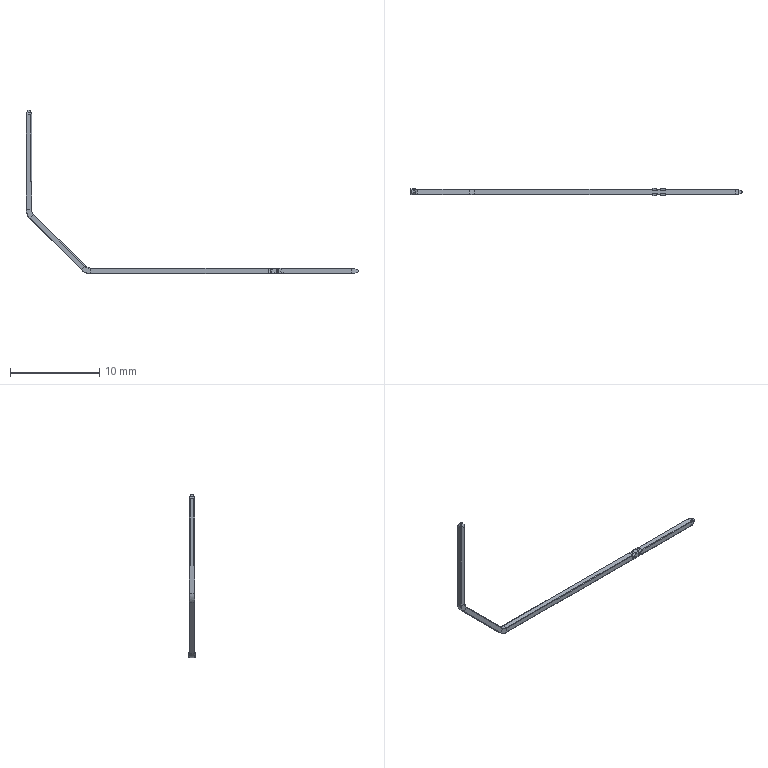Part | NX | features BREP 1 | 1 solid | 222 faces | box 37.215 x 0.8779 x 18.316 mm | volume 19.824 mm3 | cylinder 92 | plane 78 | torus 28 | sphere 20 | spline 4 | commonest cylinder face diameters 0.1 x32 0.09 x28 0.2 x12 2.01 x8 1 x4 2 x4